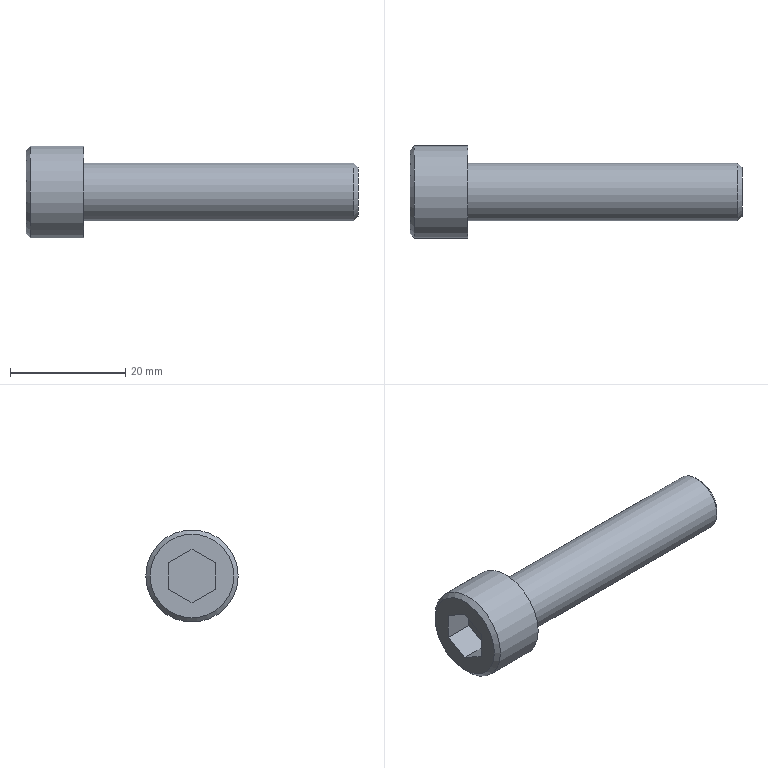Part | STEP file | solid 256 | 1 solid | 14 faces | box 57.5 x 16 x 16 mm | volume 5442 mm3 | plane 10 | cone 2 | cylinder 2 | commonest cylinder face diameters 10 x1 16 x1